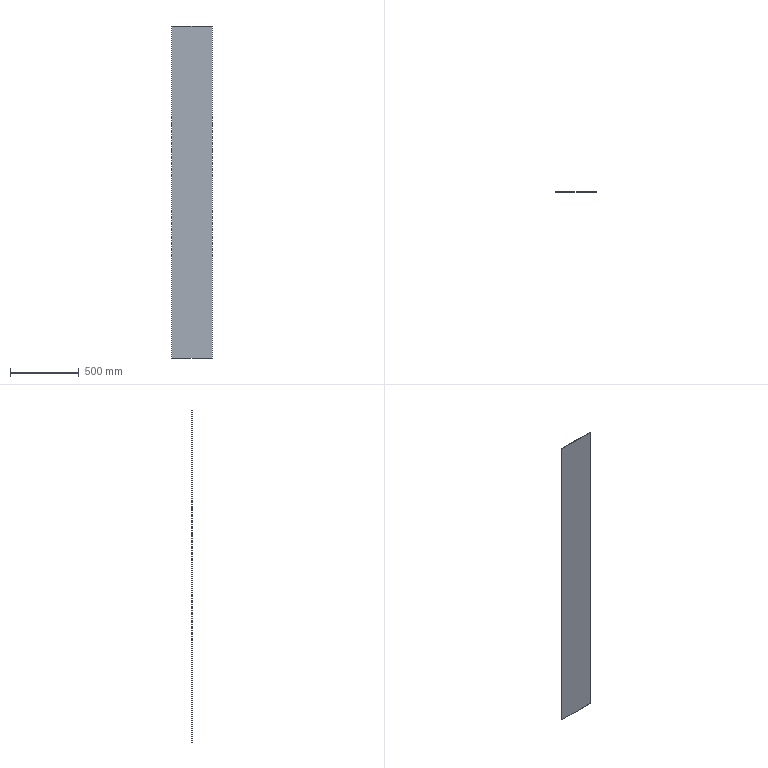Part | STEP file | E3-中转釜花纹Plate 1 | 1 solid | 6 faces | box 296 x 3 x 2420 mm | volume 2148960 mm3 | plane 6
STEP:
#1=CARTESIAN_POINT('',(0.,0.,0.));
#2=DIRECTION('',(0.,0.,1.));
#3=DIRECTION('',(1.,0.,0.));
#4=AXIS2_PLACEMENT_3D('',#1,#2,#3);
#5=CARTESIAN_POINT('',(0.,0.,2420.));
#6=VERTEX_POINT('',#5);
#7=CARTESIAN_POINT('',(0.,0.,0.));
#8=VERTEX_POINT('',#7);
#9=CARTESIAN_POINT('',(0.,0.,0.));
#10=DIRECTION('',(0.,0.,-1.));
#11=VECTOR('',#10,1.);
#12=LINE('',#9,#11);
#13=CARTESIAN_POINT('',(0.,3.,0.));
#14=DIRECTION('',(1.,0.,0.));
#15=DIRECTION('',(0.,0.,1.));
#16=AXIS2_PLACEMENT_3D('',#13,#14,#15);
#17=PLANE('',#16);
#18=CARTESIAN_POINT('',(0.,3.));
#19=DIRECTION('',(-1.,0.));
#20=VECTOR('',#19,1.);
#21=LINE('',#18,#20);
#22=(GEOMETRIC_REPRESENTATION_CONTEXT(2)PARAMETRIC_REPRESENTATION_CONTEXT()REPRESENTATION_CONTEXT('',''));
#23=DEFINITIONAL_REPRESENTATION('',(#21),#22);
#24=PCURVE('',#17,#23);
#25=CARTESIAN_POINT('',(0.,0.,0.));
#26=DIRECTION('',(0.,-1.,0.));
#27=DIRECTION('',(0.,0.,1.));
#28=AXIS2_PLACEMENT_3D('',#25,#26,#27);
#29=PLANE('',#28);
#30=CARTESIAN_POINT('',(0.,0.));
#31=DIRECTION('',(-1.,0.));
#32=VECTOR('',#31,1.);
#33=LINE('',#30,#32);
#34=(GEOMETRIC_REPRESENTATION_CONTEXT(2)PARAMETRIC_REPRESENTATION_CONTEXT()REPRESENTATION_CONTEXT('',''));
#35=DEFINITIONAL_REPRESENTATION('',(#33),#34);
#36=PCURVE('',#29,#35);
#37=SURFACE_CURVE('',#12,(#24,#36),.PCURVE_S1.);
#38=EDGE_CURVE('',#6,#8,#37,.T.);
#39=ORIENTED_EDGE('',*,*,#38,.F.);
#40=CARTESIAN_POINT('',(0.,3.,2420.));
#41=VERTEX_POINT('',#40);
#42=CARTESIAN_POINT('',(0.,3.,2420.));
#43=DIRECTION('',(0.,-1.,0.));
#44=VECTOR('',#43,1.);
#45=LINE('',#42,#44);
#46=CARTESIAN_POINT('',(2420.,0.));
#47=DIRECTION('',(0.,1.));
#48=VECTOR('',#47,1.);
#49=LINE('',#46,#48);
#50=(GEOMETRIC_REPRESENTATION_CONTEXT(2)PARAMETRIC_REPRESENTATION_CONTEXT()REPRESENTATION_CONTEXT('',''));
#51=DEFINITIONAL_REPRESENTATION('',(#49),#50);
#52=PCURVE('',#17,#51);
#53=CARTESIAN_POINT('',(0.,3.,2420.));
#54=DIRECTION('',(0.,0.,-1.));
#55=DIRECTION('',(1.,0.,0.));
#56=AXIS2_PLACEMENT_3D('',#53,#54,#55);
#57=PLANE('',#56);
#58=CARTESIAN_POINT('',(0.,0.));
#59=DIRECTION('',(0.,1.));
#60=VECTOR('',#59,1.);
#61=LINE('',#58,#60);
#62=(GEOMETRIC_REPRESENTATION_CONTEXT(2)PARAMETRIC_REPRESENTATION_CONTEXT()REPRESENTATION_CONTEXT('',''));
#63=DEFINITIONAL_REPRESENTATION('',(#61),#62);
#64=PCURVE('',#57,#63);
#65=SURFACE_CURVE('',#45,(#52,#64),.PCURVE_S1.);
#66=EDGE_CURVE('',#41,#6,#65,.T.);
#67=ORIENTED_EDGE('',*,*,#66,.F.);
#68=CARTESIAN_POINT('',(0.,3.,0.));
#69=VERTEX_POINT('',#68);
#70=CARTESIAN_POINT('',(0.,3.,0.));
#71=DIRECTION('',(0.,0.,-1.));
#72=VECTOR('',#71,1.);
#73=LINE('',#70,#72);
#74=CARTESIAN_POINT('',(0.,0.));
#75=DIRECTION('',(-1.,0.));
#76=VECTOR('',#75,1.);
#77=LINE('',#74,#76);
#78=(GEOMETRIC_REPRESENTATION_CONTEXT(2)PARAMETRIC_REPRESENTATION_CONTEXT()REPRESENTATION_CONTEXT('',''));
#79=DEFINITIONAL_REPRESENTATION('',(#77),#78);
#80=PCURVE('',#17,#79);
#81=CARTESIAN_POINT('',(0.,3.,0.));
#82=DIRECTION('',(0.,-1.,0.));
#83=DIRECTION('',(0.,0.,1.));
#84=AXIS2_PLACEMENT_3D('',#81,#82,#83);
#85=PLANE('',#84);
#86=CARTESIAN_POINT('',(0.,0.));
#87=DIRECTION('',(-1.,0.));
#88=VECTOR('',#87,1.);
#89=LINE('',#86,#88);
#90=(GEOMETRIC_REPRESENTATION_CONTEXT(2)PARAMETRIC_REPRESENTATION_CONTEXT()REPRESENTATION_CONTEXT('',''));
#91=DEFINITIONAL_REPRESENTATION('',(#89),#90);
#92=PCURVE('',#85,#91);
#93=SURFACE_CURVE('',#73,(#80,#92),.PCURVE_S1.);
#94=EDGE_CURVE('',#41,#69,#93,.T.);
#95=ORIENTED_EDGE('',*,*,#94,.T.);
#96=CARTESIAN_POINT('',(0.,3.,0.));
#97=DIRECTION('',(0.,-1.,0.));
#98=VECTOR('',#97,1.);
#99=LINE('',#96,#98);
#100=CARTESIAN_POINT('',(0.,0.));
#101=DIRECTION('',(0.,1.));
#102=VECTOR('',#101,1.);
#103=LINE('',#100,#102);
#104=(GEOMETRIC_REPRESENTATION_CONTEXT(2)PARAMETRIC_REPRESENTATION_CONTEXT()REPRESENTATION_CONTEXT('',''));
#105=DEFINITIONAL_REPRESENTATION('',(#103),#104);
#106=PCURVE('',#17,#105);
#107=CARTESIAN_POINT('',(0.,3.,0.));
#108=DIRECTION('',(0.,0.,1.));
#109=DIRECTION('',(-1.,0.,0.));
#110=AXIS2_PLACEMENT_3D('',#107,#108,#109);
#111=PLANE('',#110);
#112=CARTESIAN_POINT('',(0.,0.));
#113=DIRECTION('',(0.,1.));
#114=VECTOR('',#113,1.);
#115=LINE('',#112,#114);
#116=(GEOMETRIC_REPRESENTATION_CONTEXT(2)PARAMETRIC_REPRESENTATION_CONTEXT()REPRESENTATION_CONTEXT('',''));
#117=DEFINITIONAL_REPRESENTATION('',(#115),#116);
#118=PCURVE('',#111,#117);
#119=SURFACE_CURVE('',#99,(#106,#118),.PCURVE_S1.);
#120=EDGE_CURVE('',#69,#8,#119,.T.);
#121=ORIENTED_EDGE('',*,*,#120,.T.);
#122=EDGE_LOOP('',(#39,#67,#95,#121));
#123=FACE_BOUND('',#122,.T.);
#124=ADVANCED_FACE('',(#123),#17,.F.);
#125=CARTESIAN_POINT('',(296.,0.,0.));
#126=VERTEX_POINT('',#125);
#127=CARTESIAN_POINT('',(0.,0.,0.));
#128=DIRECTION('',(1.,0.,0.));
#129=VECTOR('',#128,1.);
#130=LINE('',#127,#129);
#131=CARTESIAN_POINT('',(0.,3.));
#132=DIRECTION('',(-1.,0.));
#133=VECTOR('',#132,1.);
#134=LINE('',#131,#133);
#135=(GEOMETRIC_REPRESENTATION_CONTEXT(2)PARAMETRIC_REPRESENTATION_CONTEXT()REPRESENTATION_CONTEXT('',''));
#136=DEFINITIONAL_REPRESENTATION('',(#134),#135);
#137=PCURVE('',#111,#136);
#138=CARTESIAN_POINT('',(0.,0.));
#139=DIRECTION('',(0.,-1.));
#140=VECTOR('',#139,1.);
#141=LINE('',#138,#140);
#142=(GEOMETRIC_REPRESENTATION_CONTEXT(2)PARAMETRIC_REPRESENTATION_CONTEXT()REPRESENTATION_CONTEXT('',''));
#143=DEFINITIONAL_REPRESENTATION('',(#141),#142);
#144=PCURVE('',#29,#143);
#145=SURFACE_CURVE('',#130,(#137,#144),.PCURVE_S1.);
#146=EDGE_CURVE('',#8,#126,#145,.T.);
#147=ORIENTED_EDGE('',*,*,#146,.F.);
#148=ORIENTED_EDGE('',*,*,#120,.F.);
#149=CARTESIAN_POINT('',(296.,3.,0.));
#150=VERTEX_POINT('',#149);
#151=CARTESIAN_POINT('',(0.,3.,0.));
#152=DIRECTION('',(1.,0.,0.));
#153=VECTOR('',#152,1.);
#154=LINE('',#151,#153);
#155=CARTESIAN_POINT('',(0.,0.));
#156=DIRECTION('',(-1.,0.));
#157=VECTOR('',#156,1.);
#158=LINE('',#155,#157);
#159=(GEOMETRIC_REPRESENTATION_CONTEXT(2)PARAMETRIC_REPRESENTATION_CONTEXT()REPRESENTATION_CONTEXT('',''));
#160=DEFINITIONAL_REPRESENTATION('',(#158),#159);
#161=PCURVE('',#111,#160);
#162=CARTESIAN_POINT('',(0.,0.));
#163=DIRECTION('',(0.,-1.));
#164=VECTOR('',#163,1.);
#165=LINE('',#162,#164);
#166=(GEOMETRIC_REPRESENTATION_CONTEXT(2)PARAMETRIC_REPRESENTATION_CONTEXT()REPRESENTATION_CONTEXT('',''));
#167=DEFINITIONAL_REPRESENTATION('',(#165),#166);
#168=PCURVE('',#85,#167);
#169=SURFACE_CURVE('',#154,(#161,#168),.PCURVE_S1.);
#170=EDGE_CURVE('',#69,#150,#169,.T.);
#171=ORIENTED_EDGE('',*,*,#170,.T.);
#172=CARTESIAN_POINT('',(296.,3.,0.));
#173=DIRECTION('',(0.,-1.,0.));
#174=VECTOR('',#173,1.);
#175=LINE('',#172,#174);
#176=CARTESIAN_POINT('',(-296.,0.));
#177=DIRECTION('',(0.,1.));
#178=VECTOR('',#177,1.);
#179=LINE('',#176,#178);
#180=(GEOMETRIC_REPRESENTATION_CONTEXT(2)PARAMETRIC_REPRESENTATION_CONTEXT()REPRESENTATION_CONTEXT('',''));
#181=DEFINITIONAL_REPRESENTATION('',(#179),#180);
#182=PCURVE('',#111,#181);
#183=CARTESIAN_POINT('',(296.,3.,0.));
#184=DIRECTION('',(-1.,0.,0.));
#185=DIRECTION('',(0.,0.,-1.));
#186=AXIS2_PLACEMENT_3D('',#183,#184,#185);
#187=PLANE('',#186);
#188=CARTESIAN_POINT('',(0.,0.));
#189=DIRECTION('',(0.,1.));
#190=VECTOR('',#189,1.);
#191=LINE('',#188,#190);
#192=(GEOMETRIC_REPRESENTATION_CONTEXT(2)PARAMETRIC_REPRESENTATION_CONTEXT()REPRESENTATION_CONTEXT('',''));
#193=DEFINITIONAL_REPRESENTATION('',(#191),#192);
#194=PCURVE('',#187,#193);
#195=SURFACE_CURVE('',#175,(#182,#194),.PCURVE_S1.);
#196=EDGE_CURVE('',#150,#126,#195,.T.);
#197=ORIENTED_EDGE('',*,*,#196,.T.);
#198=EDGE_LOOP('',(#147,#148,#171,#197));
#199=FACE_BOUND('',#198,.T.);
#200=ADVANCED_FACE('',(#199),#111,.F.);
#201=CARTESIAN_POINT('',(296.,0.,2420.));
#202=VERTEX_POINT('',#201);
#203=CARTESIAN_POINT('',(296.,0.,0.));
#204=DIRECTION('',(0.,0.,1.));
#205=VECTOR('',#204,1.);
#206=LINE('',#203,#205);
#207=CARTESIAN_POINT('',(0.,3.));
#208=DIRECTION('',(-1.,0.));
#209=VECTOR('',#208,1.);
#210=LINE('',#207,#209);
#211=(GEOMETRIC_REPRESENTATION_CONTEXT(2)PARAMETRIC_REPRESENTATION_CONTEXT()REPRESENTATION_CONTEXT('',''));
#212=DEFINITIONAL_REPRESENTATION('',(#210),#211);
#213=PCURVE('',#187,#212);
#214=CARTESIAN_POINT('',(0.,-296.));
#215=DIRECTION('',(1.,0.));
#216=VECTOR('',#215,1.);
#217=LINE('',#214,#216);
#218=(GEOMETRIC_REPRESENTATION_CONTEXT(2)PARAMETRIC_REPRESENTATION_CONTEXT()REPRESENTATION_CONTEXT('',''));
#219=DEFINITIONAL_REPRESENTATION('',(#217),#218);
#220=PCURVE('',#29,#219);
#221=SURFACE_CURVE('',#206,(#213,#220),.PCURVE_S1.);
#222=EDGE_CURVE('',#126,#202,#221,.T.);
#223=ORIENTED_EDGE('',*,*,#222,.F.);
#224=ORIENTED_EDGE('',*,*,#196,.F.);
#225=CARTESIAN_POINT('',(296.,3.,2420.));
#226=VERTEX_POINT('',#225);
#227=CARTESIAN_POINT('',(296.,3.,0.));
#228=DIRECTION('',(0.,0.,1.));
#229=VECTOR('',#228,1.);
#230=LINE('',#227,#229);
#231=CARTESIAN_POINT('',(0.,0.));
#232=DIRECTION('',(-1.,0.));
#233=VECTOR('',#232,1.);
#234=LINE('',#231,#233);
#235=(GEOMETRIC_REPRESENTATION_CONTEXT(2)PARAMETRIC_REPRESENTATION_CONTEXT()REPRESENTATION_CONTEXT('',''));
#236=DEFINITIONAL_REPRESENTATION('',(#234),#235);
#237=PCURVE('',#187,#236);
#238=CARTESIAN_POINT('',(0.,-296.));
#239=DIRECTION('',(1.,0.));
#240=VECTOR('',#239,1.);
#241=LINE('',#238,#240);
#242=(GEOMETRIC_REPRESENTATION_CONTEXT(2)PARAMETRIC_REPRESENTATION_CONTEXT()REPRESENTATION_CONTEXT('',''));
#243=DEFINITIONAL_REPRESENTATION('',(#241),#242);
#244=PCURVE('',#85,#243);
#245=SURFACE_CURVE('',#230,(#237,#244),.PCURVE_S1.);
#246=EDGE_CURVE('',#150,#226,#245,.T.);
#247=ORIENTED_EDGE('',*,*,#246,.T.);
#248=CARTESIAN_POINT('',(296.,3.,2420.));
#249=DIRECTION('',(0.,-1.,0.));
#250=VECTOR('',#249,1.);
#251=LINE('',#248,#250);
#252=CARTESIAN_POINT('',(-2420.,0.));
#253=DIRECTION('',(0.,1.));
#254=VECTOR('',#253,1.);
#255=LINE('',#252,#254);
#256=(GEOMETRIC_REPRESENTATION_CONTEXT(2)PARAMETRIC_REPRESENTATION_CONTEXT()REPRESENTATION_CONTEXT('',''));
#257=DEFINITIONAL_REPRESENTATION('',(#255),#256);
#258=PCURVE('',#187,#257);
#259=CARTESIAN_POINT('',(296.,0.));
#260=DIRECTION('',(0.,1.));
#261=VECTOR('',#260,1.);
#262=LINE('',#259,#261);
#263=(GEOMETRIC_REPRESENTATION_CONTEXT(2)PARAMETRIC_REPRESENTATION_CONTEXT()REPRESENTATION_CONTEXT('',''));
#264=DEFINITIONAL_REPRESENTATION('',(#262),#263);
#265=PCURVE('',#57,#264);
#266=SURFACE_CURVE('',#251,(#258,#265),.PCURVE_S1.);
#267=EDGE_CURVE('',#226,#202,#266,.T.);
#268=ORIENTED_EDGE('',*,*,#267,.T.);
#269=EDGE_LOOP('',(#223,#224,#247,#268));
#270=FACE_BOUND('',#269,.T.);
#271=ADVANCED_FACE('',(#270),#187,.F.);
#272=CARTESIAN_POINT('',(0.,0.,2420.));
#273=DIRECTION('',(-1.,0.,0.));
#274=VECTOR('',#273,1.);
#275=LINE('',#272,#274);
#276=CARTESIAN_POINT('',(0.,3.));
#277=DIRECTION('',(-1.,0.));
#278=VECTOR('',#277,1.);
#279=LINE('',#276,#278);
#280=(GEOMETRIC_REPRESENTATION_CONTEXT(2)PARAMETRIC_REPRESENTATION_CONTEXT()REPRESENTATION_CONTEXT('',''));
#281=DEFINITIONAL_REPRESENTATION('',(#279),#280);
#282=PCURVE('',#57,#281);
#283=CARTESIAN_POINT('',(2420.,0.));
#284=DIRECTION('',(0.,1.));
#285=VECTOR('',#284,1.);
#286=LINE('',#283,#285);
#287=(GEOMETRIC_REPRESENTATION_CONTEXT(2)PARAMETRIC_REPRESENTATION_CONTEXT()REPRESENTATION_CONTEXT('',''));
#288=DEFINITIONAL_REPRESENTATION('',(#286),#287);
#289=PCURVE('',#29,#288);
#290=SURFACE_CURVE('',#275,(#282,#289),.PCURVE_S1.);
#291=EDGE_CURVE('',#202,#6,#290,.T.);
#292=ORIENTED_EDGE('',*,*,#291,.F.);
#293=ORIENTED_EDGE('',*,*,#267,.F.);
#294=CARTESIAN_POINT('',(0.,3.,2420.));
#295=DIRECTION('',(-1.,0.,0.));
#296=VECTOR('',#295,1.);
#297=LINE('',#294,#296);
#298=CARTESIAN_POINT('',(0.,0.));
#299=DIRECTION('',(-1.,0.));
#300=VECTOR('',#299,1.);
#301=LINE('',#298,#300);
#302=(GEOMETRIC_REPRESENTATION_CONTEXT(2)PARAMETRIC_REPRESENTATION_CONTEXT()REPRESENTATION_CONTEXT('',''));
#303=DEFINITIONAL_REPRESENTATION('',(#301),#302);
#304=PCURVE('',#57,#303);
#305=CARTESIAN_POINT('',(2420.,0.));
#306=DIRECTION('',(0.,1.));
#307=VECTOR('',#306,1.);
#308=LINE('',#305,#307);
#309=(GEOMETRIC_REPRESENTATION_CONTEXT(2)PARAMETRIC_REPRESENTATION_CONTEXT()REPRESENTATION_CONTEXT('',''));
#310=DEFINITIONAL_REPRESENTATION('',(#308),#309);
#311=PCURVE('',#85,#310);
#312=SURFACE_CURVE('',#297,(#304,#311),.PCURVE_S1.);
#313=EDGE_CURVE('',#226,#41,#312,.T.);
#314=ORIENTED_EDGE('',*,*,#313,.T.);
#315=ORIENTED_EDGE('',*,*,#66,.T.);
#316=EDGE_LOOP('',(#292,#293,#314,#315));
#317=FACE_BOUND('',#316,.T.);
#318=ADVANCED_FACE('',(#317),#57,.F.);
#319=ORIENTED_EDGE('',*,*,#94,.F.);
#320=ORIENTED_EDGE('',*,*,#313,.F.);
#321=ORIENTED_EDGE('',*,*,#246,.F.);
#322=ORIENTED_EDGE('',*,*,#170,.F.);
#323=EDGE_LOOP('',(#319,#320,#321,#322));
#324=FACE_BOUND('',#323,.T.);
#325=ADVANCED_FACE('',(#324),#85,.F.);
#326=ORIENTED_EDGE('',*,*,#38,.T.);
#327=ORIENTED_EDGE('',*,*,#146,.T.);
#328=ORIENTED_EDGE('',*,*,#222,.T.);
#329=ORIENTED_EDGE('',*,*,#291,.T.);
#330=EDGE_LOOP('',(#326,#327,#328,#329));
#331=FACE_BOUND('',#330,.T.);
#332=ADVANCED_FACE('',(#331),#29,.T.);
#333=CLOSED_SHELL('',(#124,#200,#271,#318,#325,#332));
#334=MANIFOLD_SOLID_BREP('',#333);
#335=(LENGTH_UNIT()NAMED_UNIT(*)SI_UNIT(.MILLI.,.METRE.));
#336=UNCERTAINTY_MEASURE_WITH_UNIT(LENGTH_MEASURE(0.0000001),#335,'','');
#337=(NAMED_UNIT(*)PLANE_ANGLE_UNIT()SI_UNIT($,.RADIAN.));
#338=(NAMED_UNIT(*)SI_UNIT($,.STERADIAN.)SOLID_ANGLE_UNIT());
#339=(GEOMETRIC_REPRESENTATION_CONTEXT(3)GLOBAL_UNCERTAINTY_ASSIGNED_CONTEXT((#336))GLOBAL_UNIT_ASSIGNED_CONTEXT((#335,#337,#338))REPRESENTATION_CONTEXT('',''));
#340=ADVANCED_BREP_SHAPE_REPRESENTATION('',(#4,#334),#339);